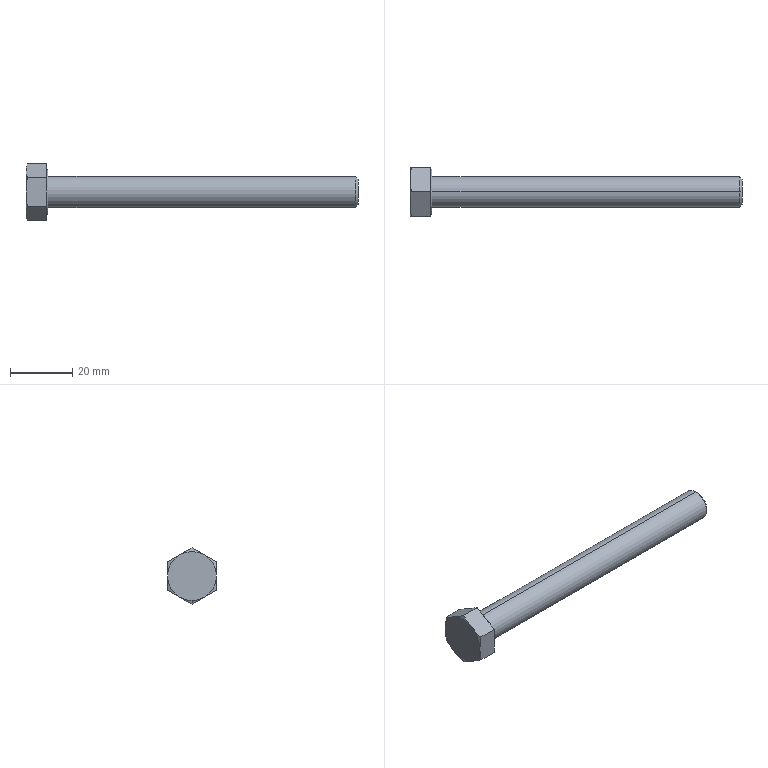Part | SolidWorks | features RevCut 2, Boss 1, Chamfer 1, Extrusion 1, Fillet 1, LPattern 1, Revolution 1 | 1 solid | 28 faces | box 107.08 x 15.73 x 18.163 mm | volume 9342 mm3 | plane 15 | cone 11 | cylinder 2 | commonest cylinder face diameters 10 x2
STEP:
#1=CARTESIAN_POINT('',(107.08,0.,-4.188));
#2=VERTEX_POINT('',#1);
#3=CARTESIAN_POINT('',(107.08,0.,4.188));
#4=VERTEX_POINT('',#3);
#5=CARTESIAN_POINT('',(107.08,0.,0.));
#6=DIRECTION('',(1.,0.,0.));
#7=DIRECTION('',(0.,0.,-1.));
#8=AXIS2_PLACEMENT_3D('',#5,#6,#7);
#9=CIRCLE('',#8,4.188);
#10=EDGE_CURVE('',#2,#4,#9,.T.);
#11=ORIENTED_EDGE('',*,*,#10,.F.);
#12=CARTESIAN_POINT('',(106.268,0.,-5.));
#13=VERTEX_POINT('',#12);
#14=CARTESIAN_POINT('',(107.08,0.,-4.188));
#15=DIRECTION('',(-0.7071,0.,-0.7071));
#16=VECTOR('',#15,1000.);
#17=LINE('',#14,#16);
#18=EDGE_CURVE('',#2,#13,#17,.T.);
#19=ORIENTED_EDGE('',*,*,#18,.T.);
#20=CARTESIAN_POINT('',(106.268,0.,5.));
#21=VERTEX_POINT('',#20);
#22=CARTESIAN_POINT('',(106.268,0.,0.));
#23=DIRECTION('',(-1.,0.,0.));
#24=DIRECTION('',(0.,0.,-1.));
#25=AXIS2_PLACEMENT_3D('',#22,#23,#24);
#26=CIRCLE('',#25,5.);
#27=EDGE_CURVE('',#21,#13,#26,.T.);
#28=ORIENTED_EDGE('',*,*,#27,.F.);
#29=CARTESIAN_POINT('',(107.08,0.,4.188));
#30=DIRECTION('',(-0.7071,0.,0.7071));
#31=VECTOR('',#30,1000.);
#32=LINE('',#29,#31);
#33=EDGE_CURVE('',#4,#21,#32,.T.);
#34=ORIENTED_EDGE('',*,*,#33,.F.);
#35=EDGE_LOOP('',(#11,#19,#28,#34));
#36=FACE_OUTER_BOUND('',#35,.T.);
#37=CARTESIAN_POINT('',(107.08,0.,0.));
#38=DIRECTION('',(-1.,0.,0.));
#39=DIRECTION('',(0.,0.,1.));
#40=AXIS2_PLACEMENT_3D('',#37,#38,#39);
#41=CONICAL_SURFACE('',#40,4.188,0.7854);
#42=ADVANCED_FACE('',(#36),#41,.T.);
#43=ORIENTED_EDGE('',*,*,#27,.T.);
#44=CARTESIAN_POINT('',(7.08,0.,-5.));
#45=VERTEX_POINT('',#44);
#46=CARTESIAN_POINT('',(107.08,0.,-5.));
#47=DIRECTION('',(-1.,0.,0.));
#48=VECTOR('',#47,1000.);
#49=LINE('',#46,#48);
#50=EDGE_CURVE('',#13,#45,#49,.T.);
#51=ORIENTED_EDGE('',*,*,#50,.T.);
#52=CARTESIAN_POINT('',(7.08,0.,5.));
#53=VERTEX_POINT('',#52);
#54=CARTESIAN_POINT('',(7.08,0.,0.));
#55=DIRECTION('',(1.,0.,0.));
#56=DIRECTION('',(0.,0.,-1.));
#57=AXIS2_PLACEMENT_3D('',#54,#55,#56);
#58=CIRCLE('',#57,5.);
#59=EDGE_CURVE('',#45,#53,#58,.T.);
#60=ORIENTED_EDGE('',*,*,#59,.T.);
#61=CARTESIAN_POINT('',(107.08,0.,5.));
#62=DIRECTION('',(-1.,0.,0.));
#63=VECTOR('',#62,1000.);
#64=LINE('',#61,#63);
#65=EDGE_CURVE('',#21,#53,#64,.T.);
#66=ORIENTED_EDGE('',*,*,#65,.F.);
#67=EDGE_LOOP('',(#43,#51,#60,#66));
#68=FACE_OUTER_BOUND('',#67,.T.);
#69=CARTESIAN_POINT('',(107.08,0.,0.));
#70=DIRECTION('',(-1.,0.,0.));
#71=DIRECTION('',(0.,0.,1.));
#72=AXIS2_PLACEMENT_3D('',#69,#70,#71);
#73=CYLINDRICAL_SURFACE('',#72,5.);
#74=ADVANCED_FACE('',(#68),#73,.T.);
#75=CARTESIAN_POINT('',(7.08,0.,7.315));
#76=VERTEX_POINT('',#75);
#77=CARTESIAN_POINT('',(7.08,0.,-7.315));
#78=VERTEX_POINT('',#77);
#79=CARTESIAN_POINT('',(7.08,0.,0.));
#80=DIRECTION('',(-1.,0.,0.));
#81=DIRECTION('',(0.,0.,1.));
#82=AXIS2_PLACEMENT_3D('',#79,#80,#81);
#83=CIRCLE('',#82,7.315);
#84=EDGE_CURVE('',#76,#78,#83,.T.);
#85=ORIENTED_EDGE('',*,*,#84,.T.);
#86=CARTESIAN_POINT('',(6.58,0.,-7.865));
#87=VERTEX_POINT('',#86);
#88=CARTESIAN_POINT('',(6.58,0.,-7.865));
#89=DIRECTION('',(-0.6727,0.,-0.7399));
#90=VECTOR('',#89,1000.);
#91=LINE('',#88,#90);
#92=EDGE_CURVE('',#78,#87,#91,.T.);
#93=ORIENTED_EDGE('',*,*,#92,.T.);
#94=CARTESIAN_POINT('',(6.58,3.933,-6.811));
#95=VERTEX_POINT('',#94);
#96=CARTESIAN_POINT('',(6.58,0.,0.));
#97=DIRECTION('',(-1.,0.,0.));
#98=DIRECTION('',(0.,0.,1.));
#99=AXIS2_PLACEMENT_3D('',#96,#97,#98);
#100=CIRCLE('',#99,7.865);
#101=EDGE_CURVE('',#95,#87,#100,.T.);
#102=ORIENTED_EDGE('',*,*,#101,.F.);
#103=CARTESIAN_POINT('',(6.58,7.865,0.));
#104=VERTEX_POINT('',#103);
#105=CARTESIAN_POINT('',(6.58,0.,0.));
#106=DIRECTION('',(-1.,0.,0.));
#107=DIRECTION('',(0.,0.,1.));
#108=AXIS2_PLACEMENT_3D('',#105,#106,#107);
#109=CIRCLE('',#108,7.865);
#110=EDGE_CURVE('',#104,#95,#109,.T.);
#111=ORIENTED_EDGE('',*,*,#110,.F.);
#112=CARTESIAN_POINT('',(6.58,3.932,6.811));
#113=VERTEX_POINT('',#112);
#114=CARTESIAN_POINT('',(6.58,0.,0.));
#115=DIRECTION('',(-1.,0.,0.));
#116=DIRECTION('',(0.,0.,1.));
#117=AXIS2_PLACEMENT_3D('',#114,#115,#116);
#118=CIRCLE('',#117,7.865);
#119=EDGE_CURVE('',#113,#104,#118,.T.);
#120=ORIENTED_EDGE('',*,*,#119,.F.);
#121=CARTESIAN_POINT('',(6.58,0.,7.865));
#122=VERTEX_POINT('',#121);
#123=CARTESIAN_POINT('',(6.58,0.,0.));
#124=DIRECTION('',(-1.,0.,0.));
#125=DIRECTION('',(0.,0.,1.));
#126=AXIS2_PLACEMENT_3D('',#123,#124,#125);
#127=CIRCLE('',#126,7.865);
#128=EDGE_CURVE('',#122,#113,#127,.T.);
#129=ORIENTED_EDGE('',*,*,#128,.F.);
#130=CARTESIAN_POINT('',(6.58,0.,7.865));
#131=DIRECTION('',(-0.6727,0.,0.7399));
#132=VECTOR('',#131,1000.);
#133=LINE('',#130,#132);
#134=EDGE_CURVE('',#76,#122,#133,.T.);
#135=ORIENTED_EDGE('',*,*,#134,.F.);
#136=EDGE_LOOP('',(#85,#93,#102,#111,#120,#129,#135));
#137=FACE_OUTER_BOUND('',#136,.T.);
#138=CARTESIAN_POINT('',(6.58,0.,0.));
#139=DIRECTION('',(-1.,0.,0.));
#140=DIRECTION('',(0.,0.,1.));
#141=AXIS2_PLACEMENT_3D('',#138,#139,#140);
#142=CONICAL_SURFACE('',#141,7.865,0.833);
#143=ADVANCED_FACE('',(#137),#142,.T.);
#144=CARTESIAN_POINT('',(0.,-3.933,-6.811));
#145=VERTEX_POINT('',#144);
#146=CARTESIAN_POINT('',(0.,0.,-7.865));
#147=VERTEX_POINT('',#146);
#148=CARTESIAN_POINT('',(0.,0.,0.));
#149=DIRECTION('',(1.,0.,0.));
#150=DIRECTION('',(0.,0.,-1.));
#151=AXIS2_PLACEMENT_3D('',#148,#149,#150);
#152=CIRCLE('',#151,7.865);
#153=EDGE_CURVE('',#145,#147,#152,.T.);
#154=ORIENTED_EDGE('',*,*,#153,.T.);
#155=CARTESIAN_POINT('',(0.4428,0.,-9.082));
#156=VERTEX_POINT('',#155);
#157=CARTESIAN_POINT('',(0.,0.,-7.865));
#158=DIRECTION('',(0.342,0.,-0.9397));
#159=VECTOR('',#158,1000.);
#160=LINE('',#157,#159);
#161=EDGE_CURVE('',#147,#156,#160,.T.);
#162=ORIENTED_EDGE('',*,*,#161,.T.);
#163=CARTESIAN_POINT('',(0.4428,0.,-9.082));
#164=CARTESIAN_POINT('',(0.3051,-0.6554,-8.703));
#165=CARTESIAN_POINT('',(0.1933,-1.311,-8.325));
#166=CARTESIAN_POINT('',(0.04049,-2.622,-7.568));
#167=CARTESIAN_POINT('',(0.,-3.277,-7.19));
#168=CARTESIAN_POINT('',(0.,-3.933,-6.811));
#169=B_SPLINE_CURVE_WITH_KNOTS('',3,(#163,#164,#165,#166,#167,#168),.UNSPECIFIED.,.F.,.F.,(4,2,4),(0.000000231,0.002271,0.004541),.UNSPECIFIED.);
#170=EDGE_CURVE('',#156,#145,#169,.T.);
#171=ORIENTED_EDGE('',*,*,#170,.T.);
#172=EDGE_LOOP('',(#154,#162,#171));
#173=FACE_OUTER_BOUND('',#172,.T.);
#174=CARTESIAN_POINT('',(0.,0.,0.));
#175=DIRECTION('',(1.,0.,0.));
#176=DIRECTION('',(0.,0.,-1.));
#177=AXIS2_PLACEMENT_3D('',#174,#175,#176);
#178=CONICAL_SURFACE('',#177,7.865,1.222);
#179=ADVANCED_FACE('',(#173),#178,.T.);
#180=ORIENTED_EDGE('',*,*,#84,.F.);
#181=CARTESIAN_POINT('',(7.08,0.,0.));
#182=DIRECTION('',(-1.,0.,0.));
#183=DIRECTION('',(0.,0.,1.));
#184=AXIS2_PLACEMENT_3D('',#181,#182,#183);
#185=CIRCLE('',#184,7.315);
#186=EDGE_CURVE('',#78,#76,#185,.T.);
#187=ORIENTED_EDGE('',*,*,#186,.F.);
#188=EDGE_LOOP('',(#180,#187));
#189=FACE_OUTER_BOUND('',#188,.T.);
#190=CARTESIAN_POINT('',(7.08,0.,0.));
#191=DIRECTION('',(1.,0.,0.));
#192=DIRECTION('',(0.,0.,-1.));
#193=AXIS2_PLACEMENT_3D('',#190,#191,#192);
#194=CIRCLE('',#193,5.);
#195=EDGE_CURVE('',#53,#45,#194,.T.);
#196=ORIENTED_EDGE('',*,*,#195,.F.);
#197=ORIENTED_EDGE('',*,*,#59,.F.);
#198=EDGE_LOOP('',(#196,#197));
#199=FACE_BOUND('',#198,.T.);
#200=CARTESIAN_POINT('',(7.08,0.,0.));
#201=DIRECTION('',(1.,0.,0.));
#202=DIRECTION('',(0.,0.,-1.));
#203=AXIS2_PLACEMENT_3D('',#200,#201,#202);
#204=PLANE('',#203);
#205=ADVANCED_FACE('',(#189,#199),#204,.T.);
#206=CARTESIAN_POINT('',(6.58,7.865,4.541));
#207=VERTEX_POINT('',#206);
#208=CARTESIAN_POINT('',(6.58,7.865,4.541));
#209=DIRECTION('',(0.,-0.866,0.5));
#210=VECTOR('',#209,1000.);
#211=LINE('',#208,#210);
#212=EDGE_CURVE('',#207,#113,#211,.T.);
#213=ORIENTED_EDGE('',*,*,#212,.T.);
#214=ORIENTED_EDGE('',*,*,#119,.T.);
#215=CARTESIAN_POINT('',(6.58,7.865,-4.541));
#216=DIRECTION('',(0.,0.,1.));
#217=VECTOR('',#216,1000.);
#218=LINE('',#215,#217);
#219=EDGE_CURVE('',#104,#207,#218,.T.);
#220=ORIENTED_EDGE('',*,*,#219,.T.);
#221=EDGE_LOOP('',(#213,#214,#220));
#222=FACE_OUTER_BOUND('',#221,.T.);
#223=CARTESIAN_POINT('',(6.58,0.,-9.082));
#224=DIRECTION('',(1.,0.,0.));
#225=DIRECTION('',(0.,0.,-1.));
#226=AXIS2_PLACEMENT_3D('',#223,#224,#225);
#227=PLANE('',#226);
#228=ADVANCED_FACE('',(#222),#227,.T.);
#229=CARTESIAN_POINT('',(6.58,7.865,-4.541));
#230=VERTEX_POINT('',#229);
#231=CARTESIAN_POINT('',(6.58,7.865,-4.541));
#232=DIRECTION('',(0.,0.,1.));
#233=VECTOR('',#232,1000.);
#234=LINE('',#231,#233);
#235=EDGE_CURVE('',#230,#104,#234,.T.);
#236=ORIENTED_EDGE('',*,*,#235,.T.);
#237=ORIENTED_EDGE('',*,*,#110,.T.);
#238=CARTESIAN_POINT('',(6.58,0.,-9.082));
#239=DIRECTION('',(0.,0.866,0.5));
#240=VECTOR('',#239,1000.);
#241=LINE('',#238,#240);
#242=EDGE_CURVE('',#95,#230,#241,.T.);
#243=ORIENTED_EDGE('',*,*,#242,.T.);
#244=EDGE_LOOP('',(#236,#237,#243));
#245=FACE_OUTER_BOUND('',#244,.T.);
#246=CARTESIAN_POINT('',(6.58,0.,-9.082));
#247=DIRECTION('',(1.,0.,0.));
#248=DIRECTION('',(0.,0.,-1.));
#249=AXIS2_PLACEMENT_3D('',#246,#247,#248);
#250=PLANE('',#249);
#251=ADVANCED_FACE('',(#245),#250,.T.);
#252=CARTESIAN_POINT('',(6.58,0.,-9.082));
#253=VERTEX_POINT('',#252);
#254=CARTESIAN_POINT('',(6.58,0.,-9.082));
#255=DIRECTION('',(0.,0.866,0.5));
#256=VECTOR('',#255,1000.);
#257=LINE('',#254,#256);
#258=EDGE_CURVE('',#253,#95,#257,.T.);
#259=ORIENTED_EDGE('',*,*,#258,.T.);
#260=ORIENTED_EDGE('',*,*,#101,.T.);
#261=CARTESIAN_POINT('',(6.58,-3.932,-6.811));
#262=VERTEX_POINT('',#261);
#263=CARTESIAN_POINT('',(6.58,0.,0.));
#264=DIRECTION('',(-1.,0.,0.));
#265=DIRECTION('',(0.,0.,1.));
#266=AXIS2_PLACEMENT_3D('',#263,#264,#265);
#267=CIRCLE('',#266,7.865);
#268=EDGE_CURVE('',#87,#262,#267,.T.);
#269=ORIENTED_EDGE('',*,*,#268,.T.);
#270=CARTESIAN_POINT('',(6.58,-7.865,-4.541));
#271=DIRECTION('',(0.,0.866,-0.5));
#272=VECTOR('',#271,1000.);
#273=LINE('',#270,#272);
#274=EDGE_CURVE('',#262,#253,#273,.T.);
#275=ORIENTED_EDGE('',*,*,#274,.T.);
#276=EDGE_LOOP('',(#259,#260,#269,#275));
#277=FACE_OUTER_BOUND('',#276,.T.);
#278=CARTESIAN_POINT('',(6.58,0.,-9.082));
#279=DIRECTION('',(1.,0.,0.));
#280=DIRECTION('',(0.,0.,-1.));
#281=AXIS2_PLACEMENT_3D('',#278,#279,#280);
#282=PLANE('',#281);
#283=ADVANCED_FACE('',(#277),#282,.T.);
#284=CARTESIAN_POINT('',(6.58,-7.865,-4.541));
#285=VERTEX_POINT('',#284);
#286=CARTESIAN_POINT('',(6.58,-7.865,-4.541));
#287=DIRECTION('',(0.,0.866,-0.5));
#288=VECTOR('',#287,1000.);
#289=LINE('',#286,#288);
#290=EDGE_CURVE('',#285,#262,#289,.T.);
#291=ORIENTED_EDGE('',*,*,#290,.T.);
#292=CARTESIAN_POINT('',(6.58,-7.865,0.));
#293=VERTEX_POINT('',#292);
#294=CARTESIAN_POINT('',(6.58,0.,0.));
#295=DIRECTION('',(-1.,0.,0.));
#296=DIRECTION('',(0.,0.,1.));
#297=AXIS2_PLACEMENT_3D('',#294,#295,#296);
#298=CIRCLE('',#297,7.865);
#299=EDGE_CURVE('',#262,#293,#298,.T.);
#300=ORIENTED_EDGE('',*,*,#299,.T.);
#301=CARTESIAN_POINT('',(6.58,-7.865,4.541));
#302=DIRECTION('',(0.,0.,-1.));
#303=VECTOR('',#302,1000.);
#304=LINE('',#301,#303);
#305=EDGE_CURVE('',#293,#285,#304,.T.);
#306=ORIENTED_EDGE('',*,*,#305,.T.);
#307=EDGE_LOOP('',(#291,#300,#306));
#308=FACE_OUTER_BOUND('',#307,.T.);
#309=CARTESIAN_POINT('',(6.58,0.,-9.082));
#310=DIRECTION('',(1.,0.,0.));
#311=DIRECTION('',(0.,0.,-1.));
#312=AXIS2_PLACEMENT_3D('',#309,#310,#311);
#313=PLANE('',#312);
#314=ADVANCED_FACE('',(#308),#313,.T.);
#315=CARTESIAN_POINT('',(6.58,-7.865,4.541));
#316=VERTEX_POINT('',#315);
#317=CARTESIAN_POINT('',(6.58,-7.865,4.541));
#318=DIRECTION('',(0.,0.,-1.));
#319=VECTOR('',#318,1000.);
#320=LINE('',#317,#319);
#321=EDGE_CURVE('',#316,#293,#320,.T.);
#322=ORIENTED_EDGE('',*,*,#321,.T.);
#323=CARTESIAN_POINT('',(6.58,-3.932,6.811));
#324=VERTEX_POINT('',#323);
#325=CARTESIAN_POINT('',(6.58,0.,0.));
#326=DIRECTION('',(-1.,0.,0.));
#327=DIRECTION('',(0.,0.,1.));
#328=AXIS2_PLACEMENT_3D('',#325,#326,#327);
#329=CIRCLE('',#328,7.865);
#330=EDGE_CURVE('',#293,#324,#329,.T.);
#331=ORIENTED_EDGE('',*,*,#330,.T.);
#332=CARTESIAN_POINT('',(6.58,0.,9.082));
#333=DIRECTION('',(0.,-0.866,-0.5));
#334=VECTOR('',#333,1000.);
#335=LINE('',#332,#334);
#336=EDGE_CURVE('',#324,#316,#335,.T.);
#337=ORIENTED_EDGE('',*,*,#336,.T.);
#338=EDGE_LOOP('',(#322,#331,#337));
#339=FACE_OUTER_BOUND('',#338,.T.);
#340=CARTESIAN_POINT('',(6.58,0.,-9.082));
#341=DIRECTION('',(1.,0.,0.));
#342=DIRECTION('',(0.,0.,-1.));
#343=AXIS2_PLACEMENT_3D('',#340,#341,#342);
#344=PLANE('',#343);
#345=ADVANCED_FACE('',(#339),#344,.T.);
#346=CARTESIAN_POINT('',(6.58,0.,9.082));
#347=VERTEX_POINT('',#346);
#348=CARTESIAN_POINT('',(6.58,0.,9.082));
#349=DIRECTION('',(0.,-0.866,-0.5));
#350=VECTOR('',#349,1000.);
#351=LINE('',#348,#350);
#352=EDGE_CURVE('',#347,#324,#351,.T.);
#353=ORIENTED_EDGE('',*,*,#352,.T.);
#354=CARTESIAN_POINT('',(6.58,0.,0.));
#355=DIRECTION('',(-1.,0.,0.));
#356=DIRECTION('',(0.,0.,1.));
#357=AXIS2_PLACEMENT_3D('',#354,#355,#356);
#358=CIRCLE('',#357,7.865);
#359=EDGE_CURVE('',#324,#122,#358,.T.);
#360=ORIENTED_EDGE('',*,*,#359,.T.);
#361=ORIENTED_EDGE('',*,*,#128,.T.);
#362=CARTESIAN_POINT('',(6.58,7.865,4.541));
#363=DIRECTION('',(0.,-0.866,0.5));
#364=VECTOR('',#363,1000.);
#365=LINE('',#362,#364);
#366=EDGE_CURVE('',#113,#347,#365,.T.);
#367=ORIENTED_EDGE('',*,*,#366,.T.);
#368=EDGE_LOOP('',(#353,#360,#361,#367));
#369=FACE_OUTER_BOUND('',#368,.T.);
#370=CARTESIAN_POINT('',(6.58,0.,-9.082));
#371=DIRECTION('',(1.,0.,0.));
#372=DIRECTION('',(0.,0.,-1.));
#373=AXIS2_PLACEMENT_3D('',#370,#371,#372);
#374=PLANE('',#373);
#375=ADVANCED_FACE('',(#369),#374,.T.);
#376=ORIENTED_EDGE('',*,*,#170,.F.);
#377=CARTESIAN_POINT('',(6.58,0.,-9.082));
#378=DIRECTION('',(-1.,0.,0.));
#379=VECTOR('',#378,1000.);
#380=LINE('',#377,#379);
#381=EDGE_CURVE('',#253,#156,#380,.T.);
#382=ORIENTED_EDGE('',*,*,#381,.F.);
#383=ORIENTED_EDGE('',*,*,#274,.F.);
#384=ORIENTED_EDGE('',*,*,#290,.F.);
#385=CARTESIAN_POINT('',(0.4428,-7.865,-4.541));
#386=VERTEX_POINT('',#385);
#387=CARTESIAN_POINT('',(6.58,-7.865,-4.541));
#388=DIRECTION('',(-1.,0.,0.));
#389=VECTOR('',#388,1000.);
#390=LINE('',#387,#389);
#391=EDGE_CURVE('',#285,#386,#390,.T.);
#392=ORIENTED_EDGE('',*,*,#391,.T.);
#393=CARTESIAN_POINT('',(0.,-3.933,-6.811));
#394=CARTESIAN_POINT('',(0.,-4.588,-6.433));
#395=CARTESIAN_POINT('',(0.04049,-5.243,-6.054));
#396=CARTESIAN_POINT('',(0.1933,-6.554,-5.298));
#397=CARTESIAN_POINT('',(0.3051,-7.21,-4.919));
#398=CARTESIAN_POINT('',(0.4428,-7.865,-4.541));
#399=B_SPLINE_CURVE_WITH_KNOTS('',3,(#393,#394,#395,#396,#397,#398),.UNSPECIFIED.,.F.,.F.,(4,2,4),(0.004541,0.006812,0.009082),.UNSPECIFIED.);
#400=EDGE_CURVE('',#145,#386,#399,.T.);
#401=ORIENTED_EDGE('',*,*,#400,.F.);
#402=EDGE_LOOP('',(#376,#382,#383,#384,#392,#401));
#403=FACE_OUTER_BOUND('',#402,.T.);
#404=CARTESIAN_POINT('',(6.58,-7.865,-4.541));
#405=DIRECTION('',(0.,0.5,0.866));
#406=DIRECTION('',(0.,-0.866,0.5));
#407=AXIS2_PLACEMENT_3D('',#404,#405,#406);
#408=PLANE('',#407);
#409=ADVANCED_FACE('',(#403),#408,.F.);
#410=CARTESIAN_POINT('',(0.4428,7.865,-4.541));
#411=VERTEX_POINT('',#410);
#412=CARTESIAN_POINT('',(0.,3.933,-6.811));
#413=VERTEX_POINT('',#412);
#414=CARTESIAN_POINT('',(0.4428,7.865,-4.541));
#415=CARTESIAN_POINT('',(0.3051,7.21,-4.919));
#416=CARTESIAN_POINT('',(0.1933,6.554,-5.298));
#417=CARTESIAN_POINT('',(0.04049,5.243,-6.054));
#418=CARTESIAN_POINT('',(0.,4.588,-6.433));
#419=CARTESIAN_POINT('',(0.,3.933,-6.811));
#420=B_SPLINE_CURVE_WITH_KNOTS('',3,(#414,#415,#416,#417,#418,#419),.UNSPECIFIED.,.F.,.F.,(4,2,4),(0.000000231,0.002271,0.004541),.UNSPECIFIED.);
#421=EDGE_CURVE('',#411,#413,#420,.T.);
#422=ORIENTED_EDGE('',*,*,#421,.F.);
#423=CARTESIAN_POINT('',(6.58,7.865,-4.541));
#424=DIRECTION('',(-1.,0.,0.));
#425=VECTOR('',#424,1000.);
#426=LINE('',#423,#425);
#427=EDGE_CURVE('',#230,#411,#426,.T.);
#428=ORIENTED_EDGE('',*,*,#427,.F.);
#429=ORIENTED_EDGE('',*,*,#242,.F.);
#430=ORIENTED_EDGE('',*,*,#258,.F.);
#431=ORIENTED_EDGE('',*,*,#381,.T.);
#432=CARTESIAN_POINT('',(0.,3.933,-6.811));
#433=CARTESIAN_POINT('',(0.,3.277,-7.19));
#434=CARTESIAN_POINT('',(0.04049,2.622,-7.568));
#435=CARTESIAN_POINT('',(0.1933,1.311,-8.325));
#436=CARTESIAN_POINT('',(0.3051,0.6554,-8.703));
#437=CARTESIAN_POINT('',(0.4428,0.,-9.082));
#438=B_SPLINE_CURVE_WITH_KNOTS('',3,(#432,#433,#434,#435,#436,#437),.UNSPECIFIED.,.F.,.F.,(4,2,4),(0.004541,0.006812,0.009082),.UNSPECIFIED.);
#439=EDGE_CURVE('',#413,#156,#438,.T.);
#440=ORIENTED_EDGE('',*,*,#439,.F.);
#441=EDGE_LOOP('',(#422,#428,#429,#430,#431,#440));
#442=FACE_OUTER_BOUND('',#441,.T.);
#443=CARTESIAN_POINT('',(6.58,0.,-9.082));
#444=DIRECTION('',(0.,-0.5,0.866));
#445=DIRECTION('',(0.,-0.866,-0.5));
#446=AXIS2_PLACEMENT_3D('',#443,#444,#445);
#447=PLANE('',#446);
#448=ADVANCED_FACE('',(#442),#447,.F.);
#449=CARTESIAN_POINT('',(0.4428,7.865,4.541));
#450=VERTEX_POINT('',#449);
#451=CARTESIAN_POINT('',(0.,7.865,0.));
#452=VERTEX_POINT('',#451);
#453=CARTESIAN_POINT('',(0.4428,7.865,4.541));
#454=CARTESIAN_POINT('',(0.3055,7.865,3.786));
#455=CARTESIAN_POINT('',(0.1936,7.865,3.029));
#456=CARTESIAN_POINT('',(0.04065,7.865,1.516));
#457=CARTESIAN_POINT('',(0.,7.865,0.7584));
#458=CARTESIAN_POINT('',(0.,7.865,0.));
#459=B_SPLINE_CURVE_WITH_KNOTS('',3,(#453,#454,#455,#456,#457,#458),.UNSPECIFIED.,.F.,.F.,(4,2,4),(0.01637,0.01866,0.02095),.UNSPECIFIED.);
#460=EDGE_CURVE('',#450,#452,#459,.T.);
#461=ORIENTED_EDGE('',*,*,#460,.F.);
#462=CARTESIAN_POINT('',(6.58,7.865,4.541));
#463=DIRECTION('',(-1.,0.,0.));
#464=VECTOR('',#463,1000.);
#465=LINE('',#462,#464);
#466=EDGE_CURVE('',#207,#450,#465,.T.);
#467=ORIENTED_EDGE('',*,*,#466,.F.);
#468=ORIENTED_EDGE('',*,*,#219,.F.);
#469=ORIENTED_EDGE('',*,*,#235,.F.);
#470=ORIENTED_EDGE('',*,*,#427,.T.);
#471=CARTESIAN_POINT('',(0.,7.865,0.));
#472=CARTESIAN_POINT('',(0.,7.865,-0.7562));
#473=CARTESIAN_POINT('',(0.04043,7.865,-1.513));
#474=CARTESIAN_POINT('',(0.1935,7.865,-3.029));
#475=CARTESIAN_POINT('',(0.306,7.865,-3.789));
#476=CARTESIAN_POINT('',(0.4428,7.865,-4.541));
#477=B_SPLINE_CURVE_WITH_KNOTS('',3,(#471,#472,#473,#474,#475,#476),.UNSPECIFIED.,.F.,.F.,(4,2,4),(0.02095,0.02323,0.02552),.UNSPECIFIED.);
#478=EDGE_CURVE('',#452,#411,#477,.T.);
#479=ORIENTED_EDGE('',*,*,#478,.F.);
#480=EDGE_LOOP('',(#461,#467,#468,#469,#470,#479));
#481=FACE_OUTER_BOUND('',#480,.T.);
#482=CARTESIAN_POINT('',(6.58,7.865,-4.541));
#483=DIRECTION('',(0.,-1.,0.));
#484=DIRECTION('',(0.,0.,-1.));
#485=AXIS2_PLACEMENT_3D('',#482,#483,#484);
#486=PLANE('',#485);
#487=ADVANCED_FACE('',(#481),#486,.F.);
#488=CARTESIAN_POINT('',(0.4428,0.,9.082));
#489=VERTEX_POINT('',#488);
#490=CARTESIAN_POINT('',(0.,3.933,6.811));
#491=VERTEX_POINT('',#490);
#492=CARTESIAN_POINT('',(0.4428,0.,9.082));
#493=CARTESIAN_POINT('',(0.3051,0.6554,8.703));
#494=CARTESIAN_POINT('',(0.1933,1.311,8.325));
#495=CARTESIAN_POINT('',(0.04049,2.622,7.568));
#496=CARTESIAN_POINT('',(0.,3.277,7.19));
#497=CARTESIAN_POINT('',(0.,3.933,6.811));
#498=B_SPLINE_CURVE_WITH_KNOTS('',3,(#492,#493,#494,#495,#496,#497),.UNSPECIFIED.,.F.,.F.,(4,2,4),(0.000000231,0.002271,0.004541),.UNSPECIFIED.);
#499=EDGE_CURVE('',#489,#491,#498,.T.);
#500=ORIENTED_EDGE('',*,*,#499,.F.);
#501=CARTESIAN_POINT('',(6.58,0.,9.082));
#502=DIRECTION('',(-1.,0.,0.));
#503=VECTOR('',#502,1000.);
#504=LINE('',#501,#503);
#505=EDGE_CURVE('',#347,#489,#504,.T.);
#506=ORIENTED_EDGE('',*,*,#505,.F.);
#507=ORIENTED_EDGE('',*,*,#366,.F.);
#508=ORIENTED_EDGE('',*,*,#212,.F.);
#509=ORIENTED_EDGE('',*,*,#466,.T.);
#510=CARTESIAN_POINT('',(0.,3.933,6.811));
#511=CARTESIAN_POINT('',(0.,4.588,6.433));
#512=CARTESIAN_POINT('',(0.04049,5.243,6.054));
#513=CARTESIAN_POINT('',(0.1933,6.554,5.298));
#514=CARTESIAN_POINT('',(0.3051,7.21,4.919));
#515=CARTESIAN_POINT('',(0.4428,7.865,4.541));
#516=B_SPLINE_CURVE_WITH_KNOTS('',3,(#510,#511,#512,#513,#514,#515),.UNSPECIFIED.,.F.,.F.,(4,2,4),(0.004541,0.006812,0.009082),.UNSPECIFIED.);
#517=EDGE_CURVE('',#491,#450,#516,.T.);
#518=ORIENTED_EDGE('',*,*,#517,.F.);
#519=EDGE_LOOP('',(#500,#506,#507,#508,#509,#518));
#520=FACE_OUTER_BOUND('',#519,.T.);
#521=CARTESIAN_POINT('',(6.58,7.865,4.541));
#522=DIRECTION('',(0.,-0.5,-0.866));
#523=DIRECTION('',(0.,0.866,-0.5));
#524=AXIS2_PLACEMENT_3D('',#521,#522,#523);
#525=PLANE('',#524);
#526=ADVANCED_FACE('',(#520),#525,.F.);
#527=CARTESIAN_POINT('',(0.4428,-7.865,4.541));
#528=VERTEX_POINT('',#527);
#529=CARTESIAN_POINT('',(0.,-3.933,6.811));
#530=VERTEX_POINT('',#529);
#531=CARTESIAN_POINT('',(0.4428,-7.865,4.541));
#532=CARTESIAN_POINT('',(0.3051,-7.21,4.919));
#533=CARTESIAN_POINT('',(0.1933,-6.554,5.298));
#534=CARTESIAN_POINT('',(0.04049,-5.243,6.054));
#535=CARTESIAN_POINT('',(0.,-4.588,6.433));
#536=CARTESIAN_POINT('',(0.,-3.933,6.811));
#537=B_SPLINE_CURVE_WITH_KNOTS('',3,(#531,#532,#533,#534,#535,#536),.UNSPECIFIED.,.F.,.F.,(4,2,4),(0.000000231,0.002271,0.004541),.UNSPECIFIED.);
#538=EDGE_CURVE('',#528,#530,#537,.T.);
#539=ORIENTED_EDGE('',*,*,#538,.F.);
#540=CARTESIAN_POINT('',(6.58,-7.865,4.541));
#541=DIRECTION('',(-1.,0.,0.));
#542=VECTOR('',#541,1000.);
#543=LINE('',#540,#542);
#544=EDGE_CURVE('',#316,#528,#543,.T.);
#545=ORIENTED_EDGE('',*,*,#544,.F.);
#546=ORIENTED_EDGE('',*,*,#336,.F.);
#547=ORIENTED_EDGE('',*,*,#352,.F.);
#548=ORIENTED_EDGE('',*,*,#505,.T.);
#549=CARTESIAN_POINT('',(0.,-3.933,6.811));
#550=CARTESIAN_POINT('',(0.,-3.277,7.19));
#551=CARTESIAN_POINT('',(0.04049,-2.622,7.568));
#552=CARTESIAN_POINT('',(0.1933,-1.311,8.325));
#553=CARTESIAN_POINT('',(0.3051,-0.6554,8.703));
#554=CARTESIAN_POINT('',(0.4428,0.,9.082));
#555=B_SPLINE_CURVE_WITH_KNOTS('',3,(#549,#550,#551,#552,#553,#554),.UNSPECIFIED.,.F.,.F.,(4,2,4),(0.004541,0.006812,0.009082),.UNSPECIFIED.);
#556=EDGE_CURVE('',#530,#489,#555,.T.);
#557=ORIENTED_EDGE('',*,*,#556,.F.);
#558=EDGE_LOOP('',(#539,#545,#546,#547,#548,#557));
#559=FACE_OUTER_BOUND('',#558,.T.);
#560=CARTESIAN_POINT('',(6.58,0.,9.082));
#561=DIRECTION('',(0.,0.5,-0.866));
#562=DIRECTION('',(0.,0.866,0.5));
#563=AXIS2_PLACEMENT_3D('',#560,#561,#562);
#564=PLANE('',#563);
#565=ADVANCED_FACE('',(#559),#564,.F.);
#566=CARTESIAN_POINT('',(0.,-7.865,0.));
#567=VERTEX_POINT('',#566);
#568=CARTESIAN_POINT('',(0.4428,-7.865,-4.541));
#569=CARTESIAN_POINT('',(0.306,-7.865,-3.789));
#570=CARTESIAN_POINT('',(0.1935,-7.865,-3.029));
#571=CARTESIAN_POINT('',(0.04043,-7.865,-1.513));
#572=CARTESIAN_POINT('',(0.,-7.865,-0.7562));
#573=CARTESIAN_POINT('',(0.,-7.865,0.));
#574=B_SPLINE_CURVE_WITH_KNOTS('',3,(#568,#569,#570,#571,#572,#573),.UNSPECIFIED.,.F.,.F.,(4,2,4),(0.007725,0.01001,0.0123),.UNSPECIFIED.);
#575=EDGE_CURVE('',#386,#567,#574,.T.);
#576=ORIENTED_EDGE('',*,*,#575,.F.);
#577=ORIENTED_EDGE('',*,*,#391,.F.);
#578=ORIENTED_EDGE('',*,*,#305,.F.);
#579=ORIENTED_EDGE('',*,*,#321,.F.);
#580=ORIENTED_EDGE('',*,*,#544,.T.);
#581=CARTESIAN_POINT('',(0.,-7.865,0.));
#582=CARTESIAN_POINT('',(0.,-7.865,0.7584));
#583=CARTESIAN_POINT('',(0.04065,-7.865,1.516));
#584=CARTESIAN_POINT('',(0.1936,-7.865,3.029));
#585=CARTESIAN_POINT('',(0.3055,-7.865,3.786));
#586=CARTESIAN_POINT('',(0.4428,-7.865,4.541));
#587=B_SPLINE_CURVE_WITH_KNOTS('',3,(#581,#582,#583,#584,#585,#586),.UNSPECIFIED.,.F.,.F.,(4,2,4),(0.0123,0.0146,0.01689),.UNSPECIFIED.);
#588=EDGE_CURVE('',#567,#528,#587,.T.);
#589=ORIENTED_EDGE('',*,*,#588,.F.);
#590=EDGE_LOOP('',(#576,#577,#578,#579,#580,#589));
#591=FACE_OUTER_BOUND('',#590,.T.);
#592=CARTESIAN_POINT('',(6.58,-7.865,4.541));
#593=DIRECTION('',(0.,1.,0.));
#594=DIRECTION('',(0.,0.,1.));
#595=AXIS2_PLACEMENT_3D('',#592,#593,#594);
#596=PLANE('',#595);
#597=ADVANCED_FACE('',(#591),#596,.F.);
#598=ORIENTED_EDGE('',*,*,#161,.F.);
#599=CARTESIAN_POINT('',(0.,0.,0.));
#600=DIRECTION('',(1.,0.,0.));
#601=DIRECTION('',(0.,0.,-1.));
#602=AXIS2_PLACEMENT_3D('',#599,#600,#601);
#603=CIRCLE('',#602,7.865);
#604=EDGE_CURVE('',#147,#413,#603,.T.);
#605=ORIENTED_EDGE('',*,*,#604,.T.);
#606=ORIENTED_EDGE('',*,*,#439,.T.);
#607=EDGE_LOOP('',(#598,#605,#606));
#608=FACE_OUTER_BOUND('',#607,.T.);
#609=CARTESIAN_POINT('',(0.,0.,0.));
#610=DIRECTION('',(1.,0.,0.));
#611=DIRECTION('',(0.,0.,-1.));
#612=AXIS2_PLACEMENT_3D('',#609,#610,#611);
#613=CONICAL_SURFACE('',#612,7.865,1.222);
#614=ADVANCED_FACE('',(#608),#613,.T.);
#615=ORIENTED_EDGE('',*,*,#400,.T.);
#616=ORIENTED_EDGE('',*,*,#575,.T.);
#617=CARTESIAN_POINT('',(0.,0.,0.));
#618=DIRECTION('',(1.,0.,0.));
#619=DIRECTION('',(0.,0.,-1.));
#620=AXIS2_PLACEMENT_3D('',#617,#618,#619);
#621=CIRCLE('',#620,7.865);
#622=EDGE_CURVE('',#567,#145,#621,.T.);
#623=ORIENTED_EDGE('',*,*,#622,.T.);
#624=EDGE_LOOP('',(#615,#616,#623));
#625=FACE_OUTER_BOUND('',#624,.T.);
#626=CARTESIAN_POINT('',(0.,0.,0.));
#627=DIRECTION('',(1.,0.,0.));
#628=DIRECTION('',(0.,0.,-1.));
#629=AXIS2_PLACEMENT_3D('',#626,#627,#628);
#630=CONICAL_SURFACE('',#629,7.865,1.222);
#631=ADVANCED_FACE('',(#625),#630,.T.);
#632=ORIENTED_EDGE('',*,*,#538,.T.);
#633=CARTESIAN_POINT('',(0.,0.,0.));
#634=DIRECTION('',(1.,0.,0.));
#635=DIRECTION('',(0.,0.,-1.));
#636=AXIS2_PLACEMENT_3D('',#633,#634,#635);
#637=CIRCLE('',#636,7.865);
#638=EDGE_CURVE('',#530,#567,#637,.T.);
#639=ORIENTED_EDGE('',*,*,#638,.T.);
#640=ORIENTED_EDGE('',*,*,#588,.T.);
#641=EDGE_LOOP('',(#632,#639,#640));
#642=FACE_OUTER_BOUND('',#641,.T.);
#643=CARTESIAN_POINT('',(0.,0.,0.));
#644=DIRECTION('',(1.,0.,0.));
#645=DIRECTION('',(0.,0.,-1.));
#646=AXIS2_PLACEMENT_3D('',#643,#644,#645);
#647=CONICAL_SURFACE('',#646,7.865,1.222);
#648=ADVANCED_FACE('',(#642),#647,.T.);
#649=ORIENTED_EDGE('',*,*,#499,.T.);
#650=CARTESIAN_POINT('',(0.,0.,0.));
#651=DIRECTION('',(1.,0.,0.));
#652=DIRECTION('',(0.,0.,-1.));
#653=AXIS2_PLACEMENT_3D('',#650,#651,#652);
#654=CIRCLE('',#653,7.865);
#655=EDGE_CURVE('',#491,#530,#654,.T.);
#656=ORIENTED_EDGE('',*,*,#655,.T.);
#657=ORIENTED_EDGE('',*,*,#556,.T.);
#658=EDGE_LOOP('',(#649,#656,#657));
#659=FACE_OUTER_BOUND('',#658,.T.);
#660=CARTESIAN_POINT('',(0.,0.,0.));
#661=DIRECTION('',(1.,0.,0.));
#662=DIRECTION('',(0.,0.,-1.));
#663=AXIS2_PLACEMENT_3D('',#660,#661,#662);
#664=CONICAL_SURFACE('',#663,7.865,1.222);
#665=ADVANCED_FACE('',(#659),#664,.T.);
#666=ORIENTED_EDGE('',*,*,#460,.T.);
#667=CARTESIAN_POINT('',(0.,0.,0.));
#668=DIRECTION('',(-1.,0.,0.));
#669=DIRECTION('',(0.,0.,1.));
#670=AXIS2_PLACEMENT_3D('',#667,#668,#669);
#671=CIRCLE('',#670,7.865);
#672=EDGE_CURVE('',#491,#452,#671,.T.);
#673=ORIENTED_EDGE('',*,*,#672,.F.);
#674=ORIENTED_EDGE('',*,*,#517,.T.);
#675=EDGE_LOOP('',(#666,#673,#674));
#676=FACE_OUTER_BOUND('',#675,.T.);
#677=CARTESIAN_POINT('',(0.,0.,0.));
#678=DIRECTION('',(1.,0.,0.));
#679=DIRECTION('',(0.,0.,-1.));
#680=AXIS2_PLACEMENT_3D('',#677,#678,#679);
#681=CONICAL_SURFACE('',#680,7.865,1.222);
#682=ADVANCED_FACE('',(#676),#681,.T.);
#683=ORIENTED_EDGE('',*,*,#478,.T.);
#684=ORIENTED_EDGE('',*,*,#421,.T.);
#685=CARTESIAN_POINT('',(0.,0.,0.));
#686=DIRECTION('',(1.,0.,0.));
#687=DIRECTION('',(0.,0.,-1.));
#688=AXIS2_PLACEMENT_3D('',#685,#686,#687);
#689=CIRCLE('',#688,7.865);
#690=EDGE_CURVE('',#413,#452,#689,.T.);
#691=ORIENTED_EDGE('',*,*,#690,.T.);
#692=EDGE_LOOP('',(#683,#684,#691));
#693=FACE_OUTER_BOUND('',#692,.T.);
#694=CARTESIAN_POINT('',(0.,0.,0.));
#695=DIRECTION('',(1.,0.,0.));
#696=DIRECTION('',(0.,0.,-1.));
#697=AXIS2_PLACEMENT_3D('',#694,#695,#696);
#698=CONICAL_SURFACE('',#697,7.865,1.222);
#699=ADVANCED_FACE('',(#693),#698,.T.);
#700=ORIENTED_EDGE('',*,*,#690,.F.);
#701=ORIENTED_EDGE('',*,*,#604,.F.);
#702=ORIENTED_EDGE('',*,*,#153,.F.);
#703=ORIENTED_EDGE('',*,*,#622,.F.);
#704=ORIENTED_EDGE('',*,*,#638,.F.);
#705=ORIENTED_EDGE('',*,*,#655,.F.);
#706=ORIENTED_EDGE('',*,*,#672,.T.);
#707=EDGE_LOOP('',(#700,#701,#702,#703,#704,#705,#706));
#708=FACE_OUTER_BOUND('',#707,.T.);
#709=CARTESIAN_POINT('',(0.,0.,-9.082));
#710=DIRECTION('',(1.,0.,0.));
#711=DIRECTION('',(0.,0.,-1.));
#712=AXIS2_PLACEMENT_3D('',#709,#710,#711);
#713=PLANE('',#712);
#714=ADVANCED_FACE('',(#708),#713,.F.);
#715=ORIENTED_EDGE('',*,*,#92,.F.);
#716=ORIENTED_EDGE('',*,*,#186,.T.);
#717=ORIENTED_EDGE('',*,*,#134,.T.);
#718=ORIENTED_EDGE('',*,*,#359,.F.);
#719=ORIENTED_EDGE('',*,*,#330,.F.);
#720=ORIENTED_EDGE('',*,*,#299,.F.);
#721=ORIENTED_EDGE('',*,*,#268,.F.);
#722=EDGE_LOOP('',(#715,#716,#717,#718,#719,#720,#721));
#723=FACE_OUTER_BOUND('',#722,.T.);
#724=CARTESIAN_POINT('',(6.58,0.,0.));
#725=DIRECTION('',(-1.,0.,0.));
#726=DIRECTION('',(0.,0.,1.));
#727=AXIS2_PLACEMENT_3D('',#724,#725,#726);
#728=CONICAL_SURFACE('',#727,7.865,0.833);
#729=ADVANCED_FACE('',(#723),#728,.T.);
#730=ORIENTED_EDGE('',*,*,#50,.F.);
#731=CARTESIAN_POINT('',(106.268,0.,0.));
#732=DIRECTION('',(-1.,0.,0.));
#733=DIRECTION('',(0.,0.,-1.));
#734=AXIS2_PLACEMENT_3D('',#731,#732,#733);
#735=CIRCLE('',#734,5.);
#736=EDGE_CURVE('',#13,#21,#735,.T.);
#737=ORIENTED_EDGE('',*,*,#736,.T.);
#738=ORIENTED_EDGE('',*,*,#65,.T.);
#739=ORIENTED_EDGE('',*,*,#195,.T.);
#740=EDGE_LOOP('',(#730,#737,#738,#739));
#741=FACE_OUTER_BOUND('',#740,.T.);
#742=CARTESIAN_POINT('',(107.08,0.,0.));
#743=DIRECTION('',(-1.,0.,0.));
#744=DIRECTION('',(0.,0.,1.));
#745=AXIS2_PLACEMENT_3D('',#742,#743,#744);
#746=CYLINDRICAL_SURFACE('',#745,5.);
#747=ADVANCED_FACE('',(#741),#746,.T.);
#748=CARTESIAN_POINT('',(107.08,0.,0.));
#749=DIRECTION('',(1.,0.,0.));
#750=DIRECTION('',(0.,0.,-1.));
#751=AXIS2_PLACEMENT_3D('',#748,#749,#750);
#752=CIRCLE('',#751,4.188);
#753=EDGE_CURVE('',#4,#2,#752,.T.);
#754=ORIENTED_EDGE('',*,*,#753,.T.);
#755=ORIENTED_EDGE('',*,*,#10,.T.);
#756=EDGE_LOOP('',(#754,#755));
#757=FACE_OUTER_BOUND('',#756,.T.);
#758=CARTESIAN_POINT('',(107.08,0.,0.));
#759=DIRECTION('',(1.,0.,0.));
#760=DIRECTION('',(0.,0.,-1.));
#761=AXIS2_PLACEMENT_3D('',#758,#759,#760);
#762=PLANE('',#761);
#763=ADVANCED_FACE('',(#757),#762,.T.);
#764=ORIENTED_EDGE('',*,*,#18,.F.);
#765=ORIENTED_EDGE('',*,*,#753,.F.);
#766=ORIENTED_EDGE('',*,*,#33,.T.);
#767=ORIENTED_EDGE('',*,*,#736,.F.);
#768=EDGE_LOOP('',(#764,#765,#766,#767));
#769=FACE_OUTER_BOUND('',#768,.T.);
#770=CARTESIAN_POINT('',(107.08,0.,0.));
#771=DIRECTION('',(-1.,0.,0.));
#772=DIRECTION('',(0.,0.,1.));
#773=AXIS2_PLACEMENT_3D('',#770,#771,#772);
#774=CONICAL_SURFACE('',#773,4.188,0.7854);
#775=ADVANCED_FACE('',(#769),#774,.T.);
#776=CLOSED_SHELL('',(#42,#74,#143,#179,#205,#228,#251,#283,#314,#345,#375,#409,#448,#487,#526,#565,#597,#614,#631,#648,#665,#682,#699,#714,#729,#747,#763,#775));
#777=MANIFOLD_SOLID_BREP('',#776);
#778=CARTESIAN_POINT('',(0.,0.,0.));
#779=DIRECTION('',(0.,0.,1.));
#780=DIRECTION('',(1.,0.,0.));
#781=AXIS2_PLACEMENT_3D('',#778,#779,#780);
#782=(LENGTH_UNIT()NAMED_UNIT(*)SI_UNIT(.MILLI.,.METRE.));
#783=UNCERTAINTY_MEASURE_WITH_UNIT(LENGTH_MEASURE(0.00001),#782,'','');
#784=(NAMED_UNIT(*)PLANE_ANGLE_UNIT()SI_UNIT($,.RADIAN.));
#785=(NAMED_UNIT(*)SI_UNIT($,.STERADIAN.)SOLID_ANGLE_UNIT());
#786=(GEOMETRIC_REPRESENTATION_CONTEXT(3)GLOBAL_UNCERTAINTY_ASSIGNED_CONTEXT((#783))GLOBAL_UNIT_ASSIGNED_CONTEXT((#782,#784,#785))REPRESENTATION_CONTEXT('',''));
#787=ADVANCED_BREP_SHAPE_REPRESENTATION('',(#777,#781),#786);